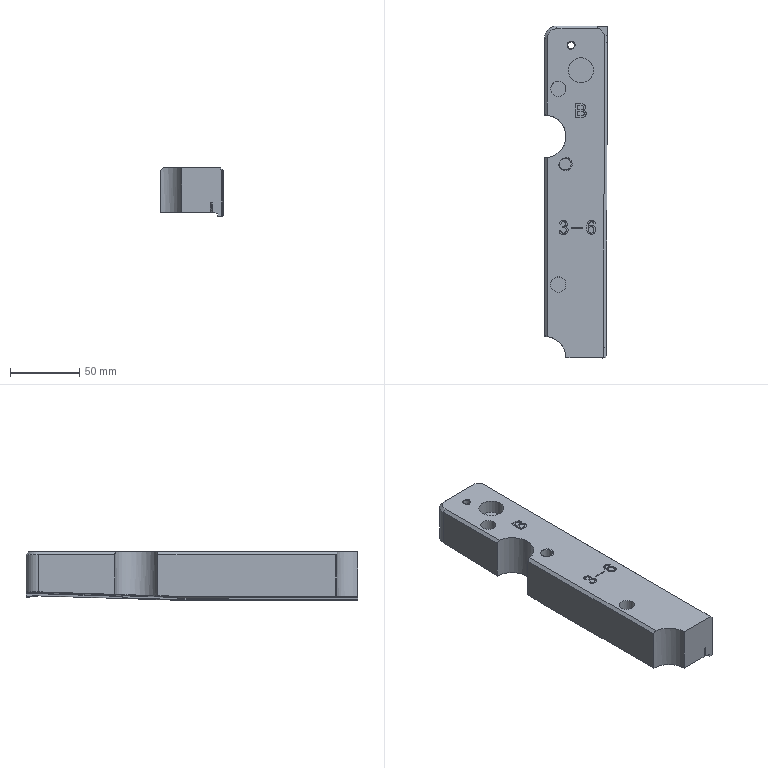NC program | NX | posted with a generic post | part box 45.476 x 239.737 x 35.001 mm
Lines 1 to 938 of 16758:
N10 G17 G21 G94 G90
(CAVITY_MILL_2 , TOOL : D16R0.8)
N12 T00 M6
N14 G53
N16 G17 G0 G90 X120.637 Y-40.184 S2500 M3
N18 G43 Z30. H0
N20 G94 G1 Z0. F4000.
N22 Z-0.2 F1380.
N24 G2 X118.8 Y-30.456 R7.
N26 G3 X121.396 Y-24.483 R17.349 F2300.
N28 X127.585 Y-22.734 R17.316
N30 G2 X136.971 Y-25.879 R7.
N32 G1 Z0.
N34 G0 Z0.3
N36 X-39.316 Y-40.181
N38 G1 Z0. F4000.
N40 Z-0.2 F1380.
N42 G2 X-41.171 Y-30.456 R7.
N44 G3 X-40.127 Y-28.705 R17.214 F2300.
N46 X-39.083 Y-30.456 R17.325
N48 G2 X-40.943 Y-40.18 R7.
N50 G1 Z0.
N52 G0 Z30.
N54 X136.069 Y-4.056
N56 G1 Z0. F4000.
N58 Z-0.2 F1380.
N60 G3 X127.585 Y-9.157 R7.
N62 G2 X119.861 Y-15.19 R7.956 F2300.
N64 G3 X112.389 Y-21.727 R7.548
N66 G2 X105.215 Y-28.632 R7.989
N68 G1 X105.033 Y-28.647
N70 G2 X103.931 Y-28.69 R14.152
N72 G1 X-24.743
N74 G2 X-32.647 Y-21.762 R7.965
N76 G3 X-47.618 Y-21.779 R7.548
N78 G2 X-54.915 Y-28.619 R7.854
N80 G1 X-55.489 Y-28.655
N82 X-55.502 Y-28.69
N84 X-110.869
N86 G2 X-125.821 Y-13.738 R14.952
N88 G1 Y16.751
N90 G2 X-123.486 Y22.367 R7.945
N92 G1 X-119.513 Y26.34
N94 G2 X-113.854 Y28.686 R8.01
N96 G1 X-107.836 Y28.69
N98 X112.158 Y27.655
N100 X112.163
N102 X119.911 Y27.614
N104 G2 X127.586 Y21.56 R7.977
N106 G3 X136.067 Y16.454 R7.
N108 G1 Z0.
N110 G0 Z0.3
N112 X120.687 Y-40.361
N114 G1 Z-0.2 F4000.
N116 Z-0.4 F1380.
N118 G2 X118.881 Y-30.628 R7.
N120 G3 X121.519 Y-24.62 R17.529 F2300.
N122 X127.759 Y-22.812 R17.464
N124 G2 X137.167 Y-25.892 R7.
N126 G1 Z-0.2
N128 G0 Z0.3
N130 X-39.276 Y-40.357
N132 G1 Z-0.2 F4000.
N134 Z-0.4 F1380.
N136 G2 X-41.101 Y-30.628 R7.
N138 G3 X-40.129 Y-29.029 R17.51 F2300.
N140 X-39.155 Y-30.628 R17.53
N142 G2 X-40.974 Y-40.358 R7.
N144 G1 Z-0.2
N146 G0 Z30.
N148 X136.161 Y-3.836
N150 G1 Z-0.2 F4000.
N152 Z-0.4 F1380.
N154 G3 X127.758 Y-9.07 R7.
N156 G2 X119.865 Y-15.338 R8.104 F2300.
N158 G3 X112.535 Y-21.75 R7.4
N160 G2 X105.196 Y-28.834 R8.169
N162 X103.931 Y-28.89 R14.352
N164 G1 X-24.748
N166 G2 X-32.797 Y-21.753 R8.17
N168 G3 X-47.468 Y-21.77 R7.4
N170 G2 X-55.515 Y-28.89 R8.15
N172 G1 X-110.869
N174 G2 X-126.021 Y-13.738 R15.152
N176 G1 Y16.537
N178 G2 X-123.592 Y22.47 R8.377
N180 G1 X-119.6 Y26.462
N182 G2 X-113.746 Y28.888 R8.283
N184 G1 X-107.836 Y28.89
N186 X112.159 Y27.855
N188 X112.164
N190 X119.911 Y27.814
N192 G2 X127.758 Y21.49 R8.167
N194 G3 X136.157 Y16.249 R7.
N196 G1 Z-0.2
N198 G0 Z0.1
N200 X120.8 Y-40.426
N202 G1 Z-0.4 F4000.
N204 Z-0.6 F1380.
N206 G2 X118.958 Y-30.699 R7.
N208 G3 X121.587 Y-24.679 R17.724 F2300.
N210 X127.828 Y-22.847 R17.56
N212 G2 X137.245 Y-25.899 R7.
N214 G1 Z-0.4
N216 G0 Z0.3
N218 X-39.143 Y-40.414
N220 G1 Z-0.4 F4000.
N222 Z-0.6 F1380.
N224 G2 X-41.045 Y-30.699 R7.
N226 G3 X-40.452 Y-29.754 R17.54 F2300.
N228 X-40.141 Y-29.199 R18.491
N230 X-39.226 Y-30.699 R17.716
N232 G2 X-41.078 Y-40.424 R7.
N234 G1 Z-0.4
N236 G0 Z30.
N238 X136.241 Y-3.857
N240 G1 Z-0.4 F4000.
N242 Z-0.6 F1380.
N244 G3 X127.829 Y-9.076 R7.
N246 G2 X120.19 Y-15.399 R8.2 F2300.
N248 G1 X119.868 Y-15.414
N250 G3 X112.61 Y-21.762 R7.324
N252 G2 X105.158 Y-29.039 R8.364
N254 X103.931 Y-29.09 R14.552
N256 G1 X-24.735
N258 G2 X-32.741 Y-22.517 R8.356
N260 G1 X-32.746 Y-22.453
N262 X-32.763 Y-22.401
N264 X-32.872 Y-21.765
N266 G3 X-47.392 Y-21.78 R7.324
N268 G2 X-48.537 Y-25.037 R9.131
N270 X-55.528 Y-29.09 R8.18
N272 G1 X-110.869
N274 G2 X-126.221 Y-13.738 R15.352
N276 G1 Y16.337
N278 G2 X-123.646 Y22.524 R9.06
N280 G1 X-119.67 Y26.5
N282 X-119.633 Y26.513
N284 X-119.447 Y26.716
N286 G2 X-113.403 Y29.09 R8.952
N288 G1 X-107.835
N290 X112.16 Y28.055
N292 X112.165
N294 X119.911 Y28.014
N296 G2 X127.829 Y21.527 R8.288
N298 G3 X136.182 Y16.214 R7.
N300 G1 Z-0.4
N302 G0 Z-0.1
N304 X120.972 Y-40.446
N306 G1 Z-0.6 F4000.
N308 Z-0.8 F1380.
N310 G2 X119.035 Y-30.737 R7.
N312 G3 X121.615 Y-24.71 R17.924 F2300.
N314 X127.867 Y-22.87 R17.558
N316 G2 X137.287 Y-25.914 R7.
N318 G1 Z-0.6
N320 G0 Z0.3
N322 X-39.002 Y-40.441
N324 G1 Z-0.6 F4000.
N326 Z-0.8 F1380.
N328 G2 X-40.962 Y-30.737 R7.
N330 G3 X-40.134 Y-29.361 R18. F2300.
N332 X-39.314 Y-30.737 R17.595
N334 G2 X-41.308 Y-40.434 R7.
N336 G1 Z-0.6
N338 G0 Z30.
N340 X136.234 Y-3.746
N342 G1 Z-0.6 F4000.
N344 Z-0.8 F1380.
N346 G3 X127.868 Y-9.039 R7.
N348 G2 X119.909 Y-15.437 R8.198 F2300.
N350 G3 X112.633 Y-21.766 R7.301
N352 G2 X107.377 Y-28.711 R8.564
N354 X105.118 Y-29.243 R8.455
N356 X103.931 Y-29.29 R14.752
N358 G1 X-24.722
N360 G2 X-32.089 Y-24.529 R8.235
N362 G1 X-32.224 Y-24.223
N364 G2 X-32.889 Y-21.825 R8.6
N366 G3 X-45.801 Y-18.14 R7.299
N368 G1 X-45.804 Y-18.144
N370 G3 X-47.403 Y-21.983 R7.442
N372 G2 X-51.309 Y-28.065 R8.64
N374 X-55.506 Y-29.29 R7.797
N376 G1 X-110.869
N378 G2 X-126.421 Y-13.738 R15.552
N380 G1 Y16.137
N382 G2 X-124.055 Y22.125 R9.133
N384 G1 X-123.751 Y22.45
N386 X-119.533 Y26.667
N388 X-119.42 Y26.775
N390 G2 X-113.114 Y29.289 R9.17
N392 G1 X-107.835 Y29.29
N394 X112.161 Y28.255
N396 X112.166
N398 X119.913 Y28.214
N400 G2 X124.994 Y26.337 R7.931
N402 X127.868 Y21.562 R8.683
N404 G3 X136.2 Y16.217 R7.
N406 G1 Z-0.6
N408 G0 Z-0.3
N410 X121.213 Y-40.417
N412 G1 Z-0.8 F4000.
N414 Z-1. F1380.
N416 G2 X119.139 Y-30.738 R7.
N418 G3 X121.634 Y-24.709 R18.03 F2300.
N420 X127.867 Y-22.871 R17.56
N422 G2 X137.287 Y-25.915 R7.
N424 G1 Z-0.8
N426 G0 Z0.3
N428 X-38.751 Y-40.411
N430 G1 Z-0.8 F4000.
N432 Z-1. F1380.
N434 G2 X-40.854 Y-30.738 R7.
N436 G3 X-40.133 Y-29.514 R18.172 F2300.
N438 X-39.562 Y-30.506 R18.303
N440 X-39.417 Y-30.738 R17.543
N442 G2 X-41.557 Y-40.403 R7.
N444 G1 Z-0.8
N446 G0 Z30.
N448 X136.236 Y-3.752
N450 G1 Z-0.8 F4000.
N452 Z-1. F1380.
N454 G3 X127.868 Y-9.042 R7.
N456 G2 X119.869 Y-15.438 R8.2 F2300.
N458 G3 X112.602 Y-22.04 R7.3
N460 G2 X108.363 Y-28.436 R8.67
N462 X105.076 Y-29.446 R8.221
N464 X103.931 Y-29.49 R14.952
N466 G1 X-24.709
N468 G2 X-31.596 Y-25.59 R8.183
N470 X-32.87 Y-21.985 R8.943
N472 G1 X-32.881 Y-21.89
N474 G3 X-47.382 Y-21.891 R7.3
N476 G2 X-50.323 Y-27.53 R8.812
N478 X-55.554 Y-29.49 R8.143
N480 G1 X-110.869
N482 G2 X-126.621 Y-13.738 R15.752
N484 G1 Y15.937
N486 G2 X-124.434 Y21.704 R9.067
N488 G1 X-123.867 Y22.336
N490 X-119.467 Y26.737
N492 G2 X-115.375 Y29.165 R9.692
N494 X-113.232 Y29.484 R7.771
N496 G1 X-112.418 Y29.49
N498 X-107.834
N500 X112.162 Y28.455
N502 X112.167
N504 X119.911 Y28.414
N506 G2 X125.853 Y25.719 R7.992
N508 X127.868 Y21.743 R8.823
N510 G3 X136.193 Y16.387 R7.
N512 G1 Z-0.8
N514 G0 Z-0.5
N516 X121.458 Y-40.387
N518 G1 Z-1. F4000.
N520 Z-1.2 F1380.
N522 G2 X119.247 Y-30.738 R7.
N524 G3 X121.652 Y-24.707 R18.085 F2300.
N526 X127.867 Y-22.871 R17.56
N528 G2 X137.287 Y-25.915 R7.
N530 G1 Z-1.
N532 G0 Z0.3
N534 X-38.478 Y-40.375
N536 G1 Z-1. F4000.
N538 Z-1.2 F1380.
N540 G2 X-40.742 Y-30.738 R7.
N542 G3 X-40.134 Y-29.678 R18.404 F2300.
N544 X-39.591 Y-30.633 R18.405
N546 G1 X-39.526 Y-30.738
N548 G2 X-41.798 Y-40.373 R7.
N550 G1 Z-1.
N552 G0 Z30.
N554 X136.236 Y-3.752
N556 G1 Z-1. F4000.
N558 Z-1.2 F1380.
N560 G3 X127.868 Y-9.042 R7.
N562 G2 X119.869 Y-15.438 R8.2 F2300.
N564 G3 X112.602 Y-22.04 R7.3
N566 G2 X109.314 Y-27.992 R8.725
N568 X105.033 Y-29.65 R8.087
N570 X103.931 Y-29.69 R15.152
N572 G1 X-24.696
N574 G2 X-31.596 Y-25.764 R8.179
N576 X-32.87 Y-21.985 R9.045
N578 G3 X-47.392 Y-21.985 R7.3
N580 G2 X-48.845 Y-26.036 R9.044
N582 X-55.567 Y-29.69 R8.134
N584 G1 X-110.869
N586 G2 X-126.821 Y-13.738 R15.952
N588 G1 Y15.737
N590 G2 X-124.845 Y21.251 R9.141
N592 G1 X-124.067 Y22.136
N594 X-119.267 Y26.937
N596 G2 X-115.89 Y29.13 R9.92
N598 X-112.418 Y29.69 R9.562
N600 G1 X-107.834
N602 X112.163 Y28.655
N604 X112.168
N606 X119.911 Y28.614
N608 G2 X127.803 Y22.236 R8.266
N610 X127.868 Y21.932 R10.442
N612 G3 X136.103 Y16.439 R7.
N614 G1 Z-1.
N616 G0 Z-0.7
N618 X121.7 Y-40.355
N620 G1 Z-1.2 F4000.
N622 Z-1.4 F1380.
N624 G2 X119.355 Y-30.738 R7.
N626 G3 X121.673 Y-24.705 R18.109 F2300.
N628 X127.867 Y-22.871 R17.56
N630 G2 X137.287 Y-25.915 R7.
N632 G1 Z-1.2
N634 G0 Z0.3
N636 X-38.223 Y-40.34
N638 G1 Z-1.2 F4000.
N640 Z-1.4 F1380.
N642 G2 X-40.631 Y-30.738 R7.
N644 G3 X-40.132 Y-29.85 R18.49 F2300.
N646 G1 X-40.131 Y-22.645
N648 X-40.132 Y-29.85
N650 G3 X-39.632 Y-30.738 R18.426
N652 G2 X-42.033 Y-40.342 R7.
N654 G1 Z-1.2
N656 G0 Z30.
N658 X136.236 Y-3.752
N660 G1 Z-1.2 F4000.
N662 Z-1.4 F1380.
N664 G3 X127.868 Y-9.042 R7.
N666 G2 X119.869 Y-15.438 R8.2 F2300.
N668 G3 X112.599 Y-22.07 R7.3
N670 G2 X109.348 Y-28.161 R8.749
N672 X104.988 Y-29.854 R8.193
N674 X103.931 Y-29.89 R15.352
N676 G1 X-24.683
N678 G2 X-31.596 Y-25.938 R8.172
N680 X-32.861 Y-22.079 R9.066
N682 G3 X-47.401 Y-22.079 R7.3
N684 G2 X-48.845 Y-26.223 R9.13
N686 X-55.58 Y-29.89 R8.168
N688 G1 X-110.869
N690 G2 X-127.021 Y-13.738 R16.152
N692 G1 Y15.537
N694 G2 X-124.875 Y21.251 R9.076
N696 G1 X-124.267 Y21.936
N698 X-119.067 Y27.137
N700 G2 X-113.403 Y29.853 R9.453
N702 G1 X-112.418 Y29.89
N704 X-107.833
N706 X112.164 Y28.855
N708 X112.17
N710 X119.911 Y28.814
N712 G2 X127.563 Y23.22 R8.189
N714 X127.868 Y22.11 R9.446
N716 G3 X136.156 Y16.696 R7.
N718 G1 Z-1.2
N720 G0 Z-0.9
N722 X121.935 Y-40.323
N724 G1 Z-1.4 F4000.
N726 Z-1.6 F1380.
N728 G2 X119.462 Y-30.738 R7.
N730 G3 X121.695 Y-24.703 R18.123 F2300.
N732 X127.867 Y-22.871 R17.56
N734 G2 X137.287 Y-25.915 R7.
N736 G1 Z-1.4
N738 G0 Z0.3
N740 X-37.985 Y-40.306
N742 G1 Z-1.4 F4000.
N744 Z-1.6 F1380.
N746 G2 X-40.522 Y-30.738 R7.
N748 G3 X-40.134 Y-30.034 R18.499 F2300.
N750 G1 X-40.131 Y-22.747
N752 X-40.134 Y-30.034
N754 G3 X-39.745 Y-30.738 R17.551
N756 G2 X-42.268 Y-40.31 R7.
N758 G1 Z-1.4
N760 G0 Z30.
N762 X136.236 Y-3.752
N764 G1 Z-1.4 F4000.
N766 Z-1.6 F1380.
N768 G3 X127.868 Y-9.041 R7.
N770 G2 X119.869 Y-15.438 R8.2 F2300.
N772 G3 X112.584 Y-22.26 R7.3
N774 G2 X109.348 Y-28.355 R8.763
N776 X105.031 Y-30.051 R7.758
N778 X103.931 Y-30.09 R15.552
N780 G1 X-24.67
N782 G2 X-32.148 Y-25.037 R8.191
N784 X-32.853 Y-22.173 R9.282
N786 G3 X-47.409 Y-22.173 R7.3
N788 G1 X-47.417 Y-22.267
N790 G2 X-48.845 Y-26.409 R9.139
N792 X-55.592 Y-30.09 R8.171
N794 G1 X-110.869
N796 G2 X-127.221 Y-13.738 R16.352
N798 G1 Y15.337
N800 G2 X-124.905 Y21.251 R9.036
N802 G1 X-124.467 Y21.736
N804 X-118.867 Y27.337
N806 G2 X-116.36 Y29.15 R10.389
N808 X-112.418 Y30.09 R9.044
N810 G1 X-107.833
N812 X112.166 Y29.055
N814 X112.171
N816 X119.911 Y29.014
N818 G2 X127.244 Y24.205 R8.142
N820 X127.868 Y22.311 R9.188
N822 G3 X136.171 Y16.92 R7.
N824 G1 Z-1.4
N826 G0 Z-1.1
N828 X122.181 Y-40.286
N830 G1 Z-1.6 F4000.
N832 Z-1.8 F1380.
N834 G2 X119.568 Y-30.738 R7.
N836 G3 X121.714 Y-24.701 R18.217 F2300.
N838 X127.867 Y-22.871 R17.56
N840 G2 X137.287 Y-25.915 R7.
N842 G1 Z-1.6
N844 G0 Z0.3
N846 X-37.797 Y-40.282
N848 G1 Z-1.6 F4000.
N850 Z-1.8 F1380.
N852 G2 X-40.424 Y-30.738 R7.
N854 G3 X-40.14 Y-30.218 R18.265 F2300.
N856 G1 X-40.131 Y-22.845
N858 X-40.14 Y-30.218
N860 G3 X-39.857 Y-30.738 R17.569
N862 G2 X-42.5 Y-40.278 R7.
N864 G1 Z-1.6
N866 G0 Z30.
N868 X136.236 Y-3.752
N870 G1 Z-1.6 F4000.
N872 Z-1.8 F1380.
N874 G3 X127.868 Y-9.041 R7.
N876 G2 X119.869 Y-15.438 R8.2 F2300.
N878 G3 X112.582 Y-22.29 R7.3
N880 G2 X110.844 Y-27.007 R8.857
N882 X104.893 Y-30.261 R8.086
N884 X103.931 Y-30.29 R15.752
N886 G1 X-24.657
N888 G2 X-32.089 Y-25.371 R8.209
N890 G1 X-32.22 Y-25.037
N892 G2 X-32.847 Y-22.267 R9.154
N894 G3 X-47.416 Y-22.267 R7.3
N896 G2 X-49.338 Y-27.26 R8.905
N898 X-55.605 Y-30.29 R8.093
N900 G1 X-110.869
N902 G2 X-127.421 Y-13.738 R16.552
N904 G1 Y15.137
N906 G2 X-124.667 Y21.536 R9.243
N908 G1 X-118.667 Y27.537
N910 G2 X-113.126 Y30.244 R9.349
N912 G1 X-112.418 Y30.289
N914 X-107.832 Y30.29
N916 X112.167 Y29.255
N918 X112.172
N920 X119.911 Y29.214
N922 G2 X127.089 Y24.736 R8.211
N924 X127.868 Y22.513 R9.24
N926 G3 X136.168 Y17.117 R7.
N928 G1 Z-1.6
N930 G0 Z-1.3
N932 X122.394 Y-40.255
N934 G1 Z-1.8 F4000.
N936 Z-2. F1380.
N938 G2 X119.671 Y-30.738 R7.
N940 G3 X121.738 Y-24.699 R18.127 F2300.
N942 X127.867 Y-22.871 R17.56
N944 G2 X137.287 Y-25.915 R7.
N946 G1 Z-1.8
N948 G0 Z0.3
N950 X-37.583 Y-40.25
N952 G1 Z-1.8 F4000.
N954 Z-2. F1380.
N956 G2 X-40.324 Y-30.738 R7.
N958 G3 X-40.141 Y-30.398 R18.217 F2300.
N960 G1 X-40.131 Y-22.942
N962 X-40.141 Y-30.398
N964 G3 X-39.96 Y-30.738 R17.566
N966 G2 X-42.727 Y-40.242 R7.
N968 G1 Z-1.8
N970 G0 Z30.
N972 X136.236 Y-3.752
N974 G1 Z-1.8 F4000.
N976 Z-2. F1380.
N978 G3 X127.868 Y-9.041 R7.
N980 G2 X119.869 Y-15.438 R8.2 F2300.
N982 G3 X112.579 Y-22.355 R7.3
N984 G2 X110.166 Y-27.992 R8.767
N986 X104.844 Y-30.464 R8.009
N988 X103.931 Y-30.49 R15.952
N990 G1 X-24.644
N992 G2 X-32.292 Y-25.037 R8.206
N994 X-32.841 Y-22.362 R9.516
N996 G3 X-47.422 Y-22.362 R7.3
N998 G2 X-49.814 Y-27.992 R8.857
N1000 X-55.618 Y-30.49 R8.088
N1002 G1 X-110.869
N1004 G2 X-127.621 Y-13.738 R16.752
N1006 G1 Y14.937
N1008 G2 X-124.867 Y21.336 R9.242
N1010 G1 X-118.467 Y27.737
N1012 G2 X-112.834 Y30.454 R9.443
N1014 G1 X-112.418 Y30.483
N1016 X-107.832 Y30.49
N1018 X112.168 Y29.455
N1020 X112.173
N1022 X119.911 Y29.414
N1024 G2 X126.131 Y26.396 R8.007
N1026 X127.868 Y22.732 R8.897
N1028 G3 X136.189 Y17.369 R7.
N1030 G1 Z-1.8
N1032 G0 Z-1.5
N1034 X122.616 Y-40.22
N1036 G1 Z-2. F4000.
N1038 Z-2.2 F1380.
N1040 G2 X119.773 Y-30.738 R7.
N1042 G3 X121.76 Y-24.696 R18.107 F2300.
N1044 X127.867 Y-22.871 R17.56
N1046 G2 X137.287 Y-25.915 R7.
N1048 G1 Z-2.
N1050 G0 Z0.3
N1052 X-37.356 Y-40.213
N1054 G1 Z-2. F4000.
N1056 Z-2.2 F1380.
N1058 G2 X-40.221 Y-30.738 R7.
N1060 G1 X-40.136 Y-30.576 F2300.
N1062 X-40.131 Y-23.039
N1064 X-40.136 Y-30.576
N1066 X-40.051 Y-30.738
N1068 G2 X-42.967 Y-40.198 R7.
N1070 G1 Z-2.
N1072 G0 Z30.
N1074 X136.236 Y-3.752
N1076 G1 Z-2. F4000.
N1078 Z-2.2 F1380.
N1080 G3 X127.868 Y-9.041 R7.
N1082 G2 X119.869 Y-15.438 R8.2 F2300.
N1084 G3 X112.574 Y-22.449 R7.3
N1086 G2 X109.348 Y-28.938 R8.747
N1088 X104.949 Y-30.658 R7.751
N1090 X103.931 Y-30.69 R16.152
N1092 G1 X-24.633
N1094 G2 X-31.61 Y-26.663 R8.058
N1096 X-32.837 Y-22.456 R9.21
N1098 G3 X-47.426 Y-22.456 R7.3
N1100 G2 X-49.634 Y-27.992 R8.879
N1102 X-55.631 Y-30.69 R8.074
N1104 G1 X-110.869
N1106 G2 X-127.821 Y-13.738 R16.952
N1108 G1 Y14.725
N1110 G2 X-125.631 Y20.5 R8.962
N1112 G1 X-125.067 Y21.136
N1114 X-118.267 Y27.937
N1116 G2 X-114.308 Y30.328 R9.818
N1118 X-111.964 Y30.69 R7.792
N1120 G1 X-107.82
N1122 X112.171 Y29.655
N1124 X119.909 Y29.614
N1126 G2 X127.089 Y25.136 R8.15
N1128 X127.866 Y22.913 R9.315
N1130 G3 X136.167 Y17.52 R7.
N1132 G1 Z-2.
N1134 G0 Z-1.7
N1136 X122.847 Y-40.179
N1138 G1 Z-2.2 F4000.
N1140 Z-2.4 F1380.
N1142 G2 X119.87 Y-30.738 R7.
N1144 G3 X121.777 Y-24.694 R18.269 F2300.
N1146 X127.867 Y-22.871 R17.56
N1148 G1 X127.868 Y-22.724
N1150 Y-9.041
N1152 G2 X119.869 Y-15.438 R8.2
N1154 G3 X112.571 Y-22.544 R7.3
N1156 G2 X110.521 Y-27.992 R8.909
N1158 X105.565 Y-30.738 R8.094
N1160 G3 X99.678 Y-38.696 R7.
N1162 G1 Z-2.2
N1164 G0 Z-1.9
N1166 X122.962 Y-40.17
N1168 G1 Z-2.4 F4000.
N1170 Z-2.6 F1380.
N1172 G2 X119.959 Y-30.737 R7.
N1174 G3 X121.809 Y-24.691 R17.639 F2300.
N1176 X127.867 Y-22.871 R17.56
N1178 G1 X127.868 Y-22.724
N1180 Y-9.041
N1182 G2 X119.869 Y-15.438 R8.2
N1184 G3 X112.569 Y-22.638 R7.3
N1186 G2 X106.391 Y-30.642 R8.279
N1188 X105.902 Y-30.738 R15.122
N1190 G3 X100.233 Y-38.853 R7.
N1192 G1 Z-2.4
N1194 G0 Z-2.1
N1196 X123.03 Y-40.159
N1198 G1 Z-2.6 F4000.
N1200 Z-2.8 F1380.
N1202 G2 X119.994 Y-30.736 R7.
N1204 G3 X121.818 Y-24.69 R17.569 F2300.
N1206 X127.867 Y-22.871 R17.56
N1208 G1 X127.868 Y-22.724
N1210 Y-9.041
N1212 G2 X119.869 Y-15.438 R8.2
N1214 G3 X112.569 Y-22.733 R7.3
N1216 G2 X106.129 Y-30.738 R8.209
N1218 G3 X100.802 Y-39.082 R7.
N1220 G1 Z-2.6
N1222 G0 Z-2.3
N1224 X123.032 Y-40.159
N1226 G1 Z-2.8 F4000.
N1228 Z-3. F1380.
N1230 G2 X119.996 Y-30.736 R7.
N1232 G3 X121.819 Y-24.69 R17.56 F2300.
N1234 X127.867 Y-22.871 R17.56
N1236 G1 X127.868 Y-22.724
N1238 Y-9.041
N1240 G2 X119.869 Y-15.438 R8.2
N1242 G3 X112.569 Y-22.733 R7.3
N1244 G2 X106.119 Y-30.738 R8.2
N1246 G3 X100.775 Y-39.071 R7.
N1248 G1 Z-2.8
N1250 G0 Z-2.5
N1252 X123.032 Y-40.159
N1254 G1 Z-3. F4000.
N1256 Z-3.2 F1380.
N1258 G2 X119.996 Y-30.736 R7.
N1260 G3 X121.819 Y-24.69 R17.56 F2300.
N1262 X127.867 Y-22.871 R17.56
N1264 G1 X127.868 Y-22.724
N1266 Y-9.041
N1268 G2 X119.869 Y-15.438 R8.2
N1270 G3 X112.569 Y-22.733 R7.3
N1272 G2 X106.119 Y-30.738 R8.2
N1274 G3 X100.775 Y-39.071 R7.
N1276 G1 Z-3.
N1278 G0 Z-2.7
N1280 X123.032 Y-40.159
N1282 G1 Z-3.2 F4000.
N1284 Z-3.4 F1380.
N1286 G2 X119.996 Y-30.736 R7.
N1288 G3 X121.819 Y-24.69 R17.56 F2300.
N1290 X127.867 Y-22.871 R17.56
N1292 G1 X127.868 Y-22.724
N1294 Y-9.041
N1296 G2 X119.869 Y-15.438 R8.2
N1298 G3 X112.569 Y-22.733 R7.3
N1300 G2 X106.119 Y-30.738 R8.2
N1302 G3 X100.775 Y-39.07 R7.
N1304 G1 Z-3.2
N1306 G0 Z-2.9
N1308 X123.032 Y-40.159
N1310 G1 Z-3.4 F4000.
N1312 Z-3.6 F1380.
N1314 G2 X119.996 Y-30.736 R7.
N1316 G3 X121.819 Y-24.69 R17.56 F2300.
N1318 X127.867 Y-22.871 R17.56
N1320 G1 X127.868 Y-22.724
N1322 Y-9.041
N1324 G2 X119.869 Y-15.438 R8.2
N1326 G3 X112.569 Y-22.733 R7.3
N1328 G2 X106.119 Y-30.738 R8.2
N1330 G3 X100.775 Y-39.07 R7.
N1332 G1 Z-3.4
N1334 G0 Z-3.1
N1336 X123.032 Y-40.159
N1338 G1 Z-3.6 F4000.
N1340 Z-3.8 F1380.
N1342 G2 X119.996 Y-30.736 R7.
N1344 G3 X121.819 Y-24.69 R17.56 F2300.
N1346 X127.867 Y-22.871 R17.56
N1348 G1 X127.868 Y-22.724
N1350 Y-9.041
N1352 G2 X119.869 Y-15.438 R8.2
N1354 G3 X112.569 Y-22.733 R7.3
N1356 G2 X106.119 Y-30.738 R8.2
N1358 G3 X100.775 Y-39.07 R7.
N1360 G1 Z-3.6
N1362 G0 Z-3.3
N1364 X123.032 Y-40.159
N1366 G1 Z-3.8 F4000.
N1368 Z-4. F1380.
N1370 G2 X119.996 Y-30.736 R7.
N1372 G3 X121.819 Y-24.69 R17.56 F2300.
N1374 X127.867 Y-22.871 R17.56
N1376 G1 X127.868 Y-22.724
N1378 Y-9.041
N1380 G2 X119.869 Y-15.438 R8.2
N1382 G3 X112.569 Y-22.733 R7.3
N1384 G2 X106.119 Y-30.738 R8.2
N1386 G3 X100.775 Y-39.07 R7.
N1388 G1 Z-3.8
N1390 G0 Z-3.5
N1392 X123.032 Y-40.159
N1394 G1 Z-4. F4000.
N1396 Z-4.2 F1380.
N1398 G2 X119.996 Y-30.736 R7.
N1400 G3 X121.819 Y-24.69 R17.56 F2300.
N1402 X127.867 Y-22.871 R17.56
N1404 G1 X127.868 Y-22.724
N1406 Y-9.041
N1408 G2 X119.869 Y-15.438 R8.2
N1410 G3 X112.569 Y-22.733 R7.3
N1412 G2 X106.119 Y-30.738 R8.2
N1414 G3 X100.775 Y-39.07 R7.
N1416 G1 Z-4.
N1418 G0 Z-3.7
N1420 X123.032 Y-40.159
N1422 G1 Z-4.2 F4000.
N1424 Z-4.4 F1380.
N1426 G2 X119.996 Y-30.736 R7.
N1428 G3 X121.819 Y-24.69 R17.56 F2300.
N1430 X127.867 Y-22.871 R17.56
N1432 G1 X127.868 Y-22.724
N1434 Y-9.041
N1436 G2 X119.869 Y-15.438 R8.2
N1438 G3 X112.569 Y-22.733 R7.3
N1440 G2 X106.119 Y-30.738 R8.2
N1442 G3 X100.775 Y-39.07 R7.
N1444 G1 Z-4.2
N1446 G0 Z-3.9
N1448 X123.032 Y-40.159
N1450 G1 Z-4.4 F4000.
N1452 Z-4.6 F1380.
N1454 G2 X119.996 Y-30.736 R7.
N1456 G3 X121.819 Y-24.69 R17.56 F2300.
N1458 X127.867 Y-22.871 R17.56
N1460 G1 X127.868 Y-22.724
N1462 Y-9.041
N1464 G2 X119.869 Y-15.438 R8.2
N1466 G3 X112.569 Y-22.733 R7.3
N1468 G2 X106.119 Y-30.738 R8.2
N1470 G3 X100.775 Y-39.07 R7.
N1472 G1 Z-4.4
N1474 G0 Z-4.1
N1476 X123.032 Y-40.159
N1478 G1 Z-4.6 F4000.
N1480 Z-4.8 F1380.
N1482 G2 X119.996 Y-30.736 R7.
N1484 G3 X121.819 Y-24.69 R17.56 F2300.
N1486 X127.867 Y-22.871 R17.56
N1488 G1 X127.868 Y-22.724
N1490 Y-9.041
N1492 G2 X119.869 Y-15.438 R8.2
N1494 G3 X112.569 Y-22.733 R7.3
N1496 G2 X106.119 Y-30.738 R8.2
N1498 G3 X100.775 Y-39.07 R7.
N1500 G1 Z-4.6
N1502 G0 Z-4.3
N1504 X123.032 Y-40.159
N1506 G1 Z-4.8 F4000.
N1508 Z-5. F1380.
N1510 G2 X119.996 Y-30.736 R7.
N1512 G3 X121.819 Y-24.69 R17.56 F2300.
N1514 X127.867 Y-22.871 R17.56
N1516 G1 X127.868 Y-22.724
N1518 Y-9.041
N1520 G2 X119.869 Y-15.438 R8.2
N1522 G3 X112.569 Y-22.733 R7.3
N1524 G2 X106.119 Y-30.738 R8.2
N1526 G3 X100.775 Y-39.07 R7.
N1528 G1 Z-4.8
N1530 G0 Z-4.5
N1532 X123.032 Y-40.159
N1534 G1 Z-5. F4000.
N1536 Z-5.2 F1380.
N1538 G2 X119.996 Y-30.736 R7.
N1540 G3 X121.819 Y-24.69 R17.56 F2300.
N1542 X127.867 Y-22.871 R17.56
N1544 G1 X127.868 Y-22.724
N1546 Y-9.041
N1548 G2 X119.869 Y-15.438 R8.2
N1550 G3 X112.569 Y-22.733 R7.3
N1552 G2 X106.119 Y-30.738 R8.2
N1554 G3 X100.774 Y-39.07 R7.
N1556 G1 Z-5.
N1558 G0 Z-4.7
N1560 X123.032 Y-40.159
N1562 G1 Z-5.2 F4000.
N1564 Z-5.4 F1380.
N1566 G2 X119.996 Y-30.736 R7.
N1568 G3 X121.819 Y-24.69 R17.56 F2300.
N1570 X127.867 Y-22.871 R17.56
N1572 G1 X127.868 Y-22.724
N1574 Y-9.041
N1576 G2 X119.869 Y-15.438 R8.2
N1578 G3 X112.569 Y-22.733 R7.3
N1580 G2 X106.119 Y-30.738 R8.2
N1582 G3 X100.774 Y-39.07 R7.
N1584 G1 Z-5.2
N1586 G0 Z-4.9
N1588 X123.032 Y-40.159
N1590 G1 Z-5.4 F4000.
N1592 Z-5.6 F1380.
N1594 G2 X119.996 Y-30.736 R7.
N1596 G3 X121.819 Y-24.69 R17.56 F2300.
N1598 X127.867 Y-22.871 R17.56
N1600 G1 X127.868 Y-22.724
N1602 Y-9.041
N1604 G2 X119.869 Y-15.438 R8.2
N1606 G3 X112.569 Y-22.733 R7.3
N1608 G2 X106.119 Y-30.738 R8.2
N1610 G3 X100.774 Y-39.07 R7.
N1612 G1 Z-5.4
N1614 G0 Z-5.1
N1616 X123.032 Y-40.159
N1618 G1 Z-5.6 F4000.
N1620 Z-5.8 F1380.
N1622 G2 X119.996 Y-30.736 R7.
N1624 G3 X121.819 Y-24.69 R17.56 F2300.
N1626 X127.867 Y-22.871 R17.56
N1628 G1 X127.868 Y-22.724
N1630 Y-9.041
N1632 G2 X119.869 Y-15.438 R8.2
N1634 G3 X112.569 Y-22.733 R7.3
N1636 G2 X106.119 Y-30.738 R8.2
N1638 G3 X100.774 Y-39.07 R7.
N1640 G1 Z-5.6
N1642 G0 Z-5.3
N1644 X123.032 Y-40.159
N1646 G1 Z-5.8 F4000.
N1648 Z-6. F1380.
N1650 G2 X119.996 Y-30.736 R7.
N1652 G3 X121.819 Y-24.69 R17.56 F2300.
N1654 X127.867 Y-22.871 R17.56
N1656 G1 X127.868 Y-22.724
N1658 Y-9.041
N1660 G2 X119.869 Y-15.438 R8.2
N1662 G3 X112.569 Y-22.733 R7.3
N1664 G2 X106.119 Y-30.738 R8.2
N1666 G3 X100.774 Y-39.07 R7.
N1668 G1 Z-5.8
N1670 G0 Z-5.5
N1672 X123.032 Y-40.159
N1674 G1 Z-6. F4000.
N1676 Z-6.2 F1380.
N1678 G2 X119.996 Y-30.736 R7.
N1680 G3 X121.819 Y-24.69 R17.56 F2300.
N1682 X127.867 Y-22.871 R17.56
N1684 G1 X127.868 Y-22.724
N1686 Y-9.041
N1688 G2 X119.869 Y-15.438 R8.2
N1690 G3 X112.569 Y-22.733 R7.3
N1692 G2 X106.119 Y-30.738 R8.2
N1694 G3 X100.774 Y-39.07 R7.
N1696 G1 Z-6.
N1698 G0 Z-5.7
N1700 X123.032 Y-40.159
N1702 G1 Z-6.2 F4000.
N1704 Z-6.4 F1380.
N1706 G2 X119.995 Y-30.736 R7.
N1708 G3 X121.819 Y-24.69 R17.56 F2300.
N1710 X127.867 Y-22.871 R17.56
N1712 G1 X127.868 Y-22.724
N1714 Y-9.041
N1716 G2 X119.869 Y-15.438 R8.2
N1718 G3 X112.569 Y-22.733 R7.3
N1720 G2 X106.119 Y-30.738 R8.2
N1722 G3 X100.774 Y-39.07 R7.
N1724 G1 Z-6.2
N1726 G0 Z-5.9
N1728 X123.032 Y-40.159
N1730 G1 Z-6.4 F4000.
N1732 Z-6.6 F1380.
N1734 G2 X119.995 Y-30.736 R7.
N1736 G3 X121.819 Y-24.69 R17.56 F2300.
N1738 X127.867 Y-22.871 R17.56
N1740 G1 X127.868 Y-22.724
N1742 Y-9.041
N1744 G2 X119.869 Y-15.438 R8.2
N1746 G3 X112.569 Y-22.733 R7.3
N1748 G2 X106.119 Y-30.738 R8.2
N1750 G3 X100.774 Y-39.07 R7.
N1752 G1 Z-6.4
N1754 G0 Z-6.1
N1756 X123.032 Y-40.159
N1758 G1 Z-6.6 F4000.
N1760 Z-6.8 F1380.
N1762 G2 X119.995 Y-30.736 R7.
N1764 G3 X121.819 Y-24.69 R17.56 F2300.
N1766 X127.867 Y-22.871 R17.56
N1768 G1 X127.868 Y-22.724
N1770 Y-9.041
N1772 G2 X119.869 Y-15.438 R8.2
N1774 G3 X112.569 Y-22.733 R7.3
N1776 G2 X106.119 Y-30.738 R8.2
N1778 G3 X100.774 Y-39.07 R7.
N1780 G1 Z-6.6
N1782 G0 Z-6.3
N1784 X123.032 Y-40.159
N1786 G1 Z-6.8 F4000.
N1788 Z-7. F1380.
N1790 G2 X119.995 Y-30.736 R7.
N1792 G3 X121.819 Y-24.69 R17.56 F2300.
N1794 X127.867 Y-22.871 R17.56
N1796 G1 X127.868 Y-22.724
N1798 Y-9.041
N1800 G2 X119.869 Y-15.438 R8.2
N1802 G3 X112.569 Y-22.733 R7.3
N1804 G2 X106.119 Y-30.738 R8.2
N1806 G3 X100.774 Y-39.07 R7.
N1808 G1 Z-6.8
N1810 G0 Z-6.5
N1812 X123.032 Y-40.159
N1814 G1 Z-7. F4000.
N1816 Z-7.2 F1380.
N1818 G2 X119.995 Y-30.736 R7.
N1820 G3 X121.819 Y-24.69 R17.56 F2300.
N1822 X127.867 Y-22.871 R17.56
N1824 G1 X127.868 Y-22.724
N1826 Y-9.041
N1828 G2 X119.869 Y-15.438 R8.2
N1830 G3 X112.569 Y-22.733 R7.3
N1832 G2 X106.119 Y-30.738 R8.2
N1834 G3 X100.774 Y-39.07 R7.
N1836 G1 Z-7.
N1838 G0 Z-6.7
N1840 X123.032 Y-40.159
N1842 G1 Z-7.2 F4000.
N1844 Z-7.4 F1380.
N1846 G2 X119.995 Y-30.736 R7.
N1848 G3 X121.819 Y-24.69 R17.56 F2300.
N1850 X127.867 Y-22.871 R17.56
N1852 G1 X127.868 Y-22.724
N1854 Y-9.041
N1856 G2 X119.869 Y-15.438 R8.2
N1858 G3 X112.569 Y-22.733 R7.3
N1860 G2 X106.119 Y-30.738 R8.2
N1862 G3 X100.774 Y-39.07 R7.
N1864 G1 Z-7.2
N1866 G0 Z-6.9
N1868 X123.032 Y-40.159
N1870 G1 Z-7.4 F4000.
N1872 Z-7.6 F1380.
N1874 G2 X119.995 Y-30.736 R7.